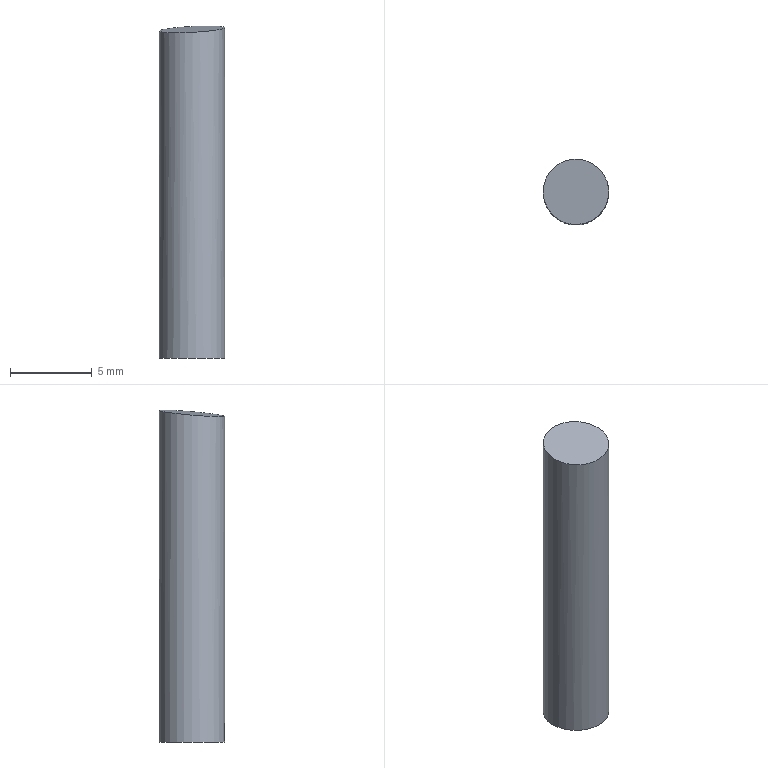Part | NX | features solid 2 | 1 solid | 3 faces | box 4 x 4 x 20.248 mm | volume 251.843 mm3 | plane 2 | cylinder 1 | commonest cylinder face diameters 4 x1
STEP:
#1=CARTESIAN_POINT('',(-192.896,7.523,-24.));
#2=VERTEX_POINT('',#1);
#3=CARTESIAN_POINT('',(-190.896,7.523,-24.));
#4=DIRECTION('',(0.,0.,-1.));
#5=DIRECTION('',(-1.,0.,0.));
#6=AXIS2_PLACEMENT_3D('',#3,#4,#5);
#7=CIRCLE('',#6,2.);
#8=EDGE_CURVE('',#2,#2,#7,.F.);
#9=ORIENTED_EDGE('',*,*,#8,.F.);
#10=EDGE_LOOP('',(#9));
#11=FACE_BOUND('',#10,.T.);
#12=CARTESIAN_POINT('',(-190.896,-11.477,-24.));
#13=DIRECTION('',(0.,0.,-1.));
#14=DIRECTION('',(-1.,0.,0.));
#15=AXIS2_PLACEMENT_3D('',#12,#13,#14);
#16=PLANE('',#15);
#17=ADVANCED_FACE('',(#11),#16,.T.);
#18=CARTESIAN_POINT('',(-191.906,5.796,-4.166));
#19=VERTEX_POINT('',#18);
#20=CARTESIAN_POINT('',(-190.896,7.523,-3.959));
#21=DIRECTION('',(0.05204,0.08903,-0.9947));
#22=DIRECTION('',(-0.502,-0.8587,-0.1031));
#23=AXIS2_PLACEMENT_3D('',#20,#21,#22);
#24=ELLIPSE('',#23,2.011,2.);
#25=EDGE_CURVE('',#19,#19,#24,.T.);
#26=ORIENTED_EDGE('',*,*,#25,.F.);
#27=EDGE_LOOP('',(#26));
#28=FACE_BOUND('',#27,.T.);
#29=CARTESIAN_POINT('',(-99.272,-11.445,-0.8629));
#30=DIRECTION('',(0.05204,0.08903,-0.9947));
#31=DIRECTION('',(0.005002,-0.996,-0.08889));
#32=AXIS2_PLACEMENT_3D('',#29,#30,#31);
#33=PLANE('',#32);
#34=ADVANCED_FACE('',(#28),#33,.F.);
#35=ORIENTED_EDGE('',*,*,#8,.T.);
#36=EDGE_LOOP('',(#35));
#37=FACE_BOUND('',#36,.T.);
#38=ORIENTED_EDGE('',*,*,#25,.T.);
#39=EDGE_LOOP('',(#38));
#40=FACE_BOUND('',#39,.T.);
#41=CARTESIAN_POINT('',(-190.896,7.523,-3.5));
#42=DIRECTION('',(0.,0.,-1.));
#43=DIRECTION('',(-1.,0.,0.));
#44=AXIS2_PLACEMENT_3D('',#41,#42,#43);
#45=CYLINDRICAL_SURFACE('',#44,2.);
#46=ADVANCED_FACE('',(#37,#40),#45,.T.);
#47=CLOSED_SHELL('',(#17,#34,#46));
#48=MANIFOLD_SOLID_BREP('',#47);
#49=(LENGTH_UNIT()NAMED_UNIT(*)SI_UNIT(.MILLI.,.METRE.));
#50=UNCERTAINTY_MEASURE_WITH_UNIT(LENGTH_MEASURE(0.00001),#49,'','');
#51=(NAMED_UNIT(*)PLANE_ANGLE_UNIT()SI_UNIT($,.RADIAN.));
#52=(NAMED_UNIT(*)SI_UNIT($,.STERADIAN.)SOLID_ANGLE_UNIT());
#53=(GEOMETRIC_REPRESENTATION_CONTEXT(3)GLOBAL_UNCERTAINTY_ASSIGNED_CONTEXT((#50))GLOBAL_UNIT_ASSIGNED_CONTEXT((#49,#51,#52))REPRESENTATION_CONTEXT('',''));
#54=ADVANCED_BREP_SHAPE_REPRESENTATION('',(#48),#53);